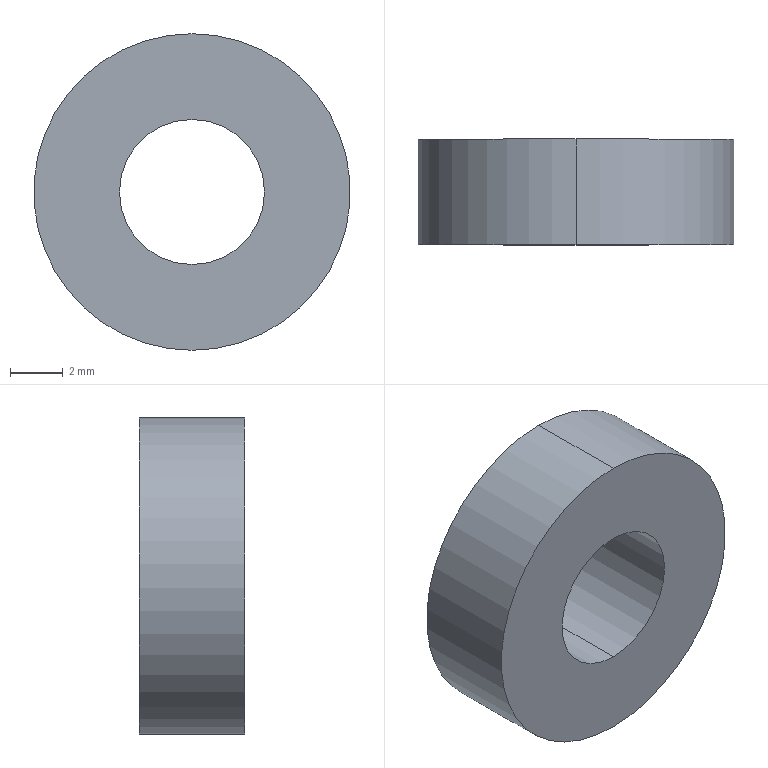Part | STEP file | PN_0026 lifting mechanism plate_Default | 1 solid | 6 faces | box 12 x 4 x 12 mm | volume 357.356 mm3 | cylinder 4 | plane 2 | commonest cylinder face diameters 5.5 x2 12 x2
STEP:
#1=CARTESIAN_POINT('',(0.,0.,0.));
#2=DIRECTION('',(0.,0.,1.));
#3=DIRECTION('',(1.,0.,0.));
#4=AXIS2_PLACEMENT_3D('',#1,#2,#3);
#5=CARTESIAN_POINT('',(0.,4.,-2.75));
#6=VERTEX_POINT('',#5);
#7=CARTESIAN_POINT('',(0.,0.,-2.75));
#8=VERTEX_POINT('',#7);
#9=CARTESIAN_POINT('',(0.,4.,-2.75));
#10=DIRECTION('',(0.,-1.,0.));
#11=VECTOR('',#10,1.);
#12=LINE('',#9,#11);
#13=CARTESIAN_POINT('',(0.,4.,0.));
#14=DIRECTION('',(0.,-1.,0.));
#15=DIRECTION('',(0.,0.,-1.));
#16=AXIS2_PLACEMENT_3D('',#13,#14,#15);
#17=CYLINDRICAL_SURFACE('',#16,2.75);
#18=CARTESIAN_POINT('',(6.283,0.));
#19=DIRECTION('',(0.,1.));
#20=VECTOR('',#19,1.);
#21=LINE('',#18,#20);
#22=(GEOMETRIC_REPRESENTATION_CONTEXT(2)PARAMETRIC_REPRESENTATION_CONTEXT()REPRESENTATION_CONTEXT('',''));
#23=DEFINITIONAL_REPRESENTATION('',(#21),#22);
#24=PCURVE('',#17,#23);
#25=CARTESIAN_POINT('',(0.,4.,0.));
#26=DIRECTION('',(0.,-1.,0.));
#27=DIRECTION('',(0.,0.,-1.));
#28=AXIS2_PLACEMENT_3D('',#25,#26,#27);
#29=CYLINDRICAL_SURFACE('',#28,2.75);
#30=CARTESIAN_POINT('',(0.,0.));
#31=DIRECTION('',(0.,1.));
#32=VECTOR('',#31,1.);
#33=LINE('',#30,#32);
#34=(GEOMETRIC_REPRESENTATION_CONTEXT(2)PARAMETRIC_REPRESENTATION_CONTEXT()REPRESENTATION_CONTEXT('',''));
#35=DEFINITIONAL_REPRESENTATION('',(#33),#34);
#36=PCURVE('',#29,#35);
#37=SURFACE_CURVE('',#12,(#24,#36),.PCURVE_S1.);
#38=EDGE_CURVE('',#6,#8,#37,.T.);
#39=ORIENTED_EDGE('',*,*,#38,.T.);
#40=CARTESIAN_POINT('',(0.,0.,2.75));
#41=VERTEX_POINT('',#40);
#42=CARTESIAN_POINT('',(0.,0.,0.));
#43=DIRECTION('',(0.,1.,0.));
#44=DIRECTION('',(0.,0.,1.));
#45=AXIS2_PLACEMENT_3D('',#42,#43,#44);
#46=CIRCLE('',#45,2.75);
#47=CARTESIAN_POINT('',(9.425,4.));
#48=DIRECTION('',(-1.,0.));
#49=VECTOR('',#48,1.);
#50=LINE('',#47,#49);
#51=(GEOMETRIC_REPRESENTATION_CONTEXT(2)PARAMETRIC_REPRESENTATION_CONTEXT()REPRESENTATION_CONTEXT('',''));
#52=DEFINITIONAL_REPRESENTATION('',(#50),#51);
#53=PCURVE('',#17,#52);
#54=CARTESIAN_POINT('',(0.,0.,0.));
#55=DIRECTION('',(0.,1.,0.));
#56=DIRECTION('',(0.,0.,1.));
#57=AXIS2_PLACEMENT_3D('',#54,#55,#56);
#58=PLANE('',#57);
#59=CARTESIAN_POINT('',(0.,0.));
#60=DIRECTION('',(1.,0.));
#61=AXIS2_PLACEMENT_2D('',#59,#60);
#62=CIRCLE('',#61,2.75);
#63=(GEOMETRIC_REPRESENTATION_CONTEXT(2)PARAMETRIC_REPRESENTATION_CONTEXT()REPRESENTATION_CONTEXT('',''));
#64=DEFINITIONAL_REPRESENTATION('',(#62),#63);
#65=PCURVE('',#58,#64);
#66=SURFACE_CURVE('',#46,(#53,#65),.PCURVE_S1.);
#67=EDGE_CURVE('',#8,#41,#66,.T.);
#68=ORIENTED_EDGE('',*,*,#67,.T.);
#69=CARTESIAN_POINT('',(0.,4.,2.75));
#70=VERTEX_POINT('',#69);
#71=CARTESIAN_POINT('',(0.,4.,2.75));
#72=DIRECTION('',(0.,-1.,0.));
#73=VECTOR('',#72,1.);
#74=LINE('',#71,#73);
#75=CARTESIAN_POINT('',(3.142,0.));
#76=DIRECTION('',(0.,1.));
#77=VECTOR('',#76,1.);
#78=LINE('',#75,#77);
#79=(GEOMETRIC_REPRESENTATION_CONTEXT(2)PARAMETRIC_REPRESENTATION_CONTEXT()REPRESENTATION_CONTEXT('',''));
#80=DEFINITIONAL_REPRESENTATION('',(#78),#79);
#81=PCURVE('',#17,#80);
#82=CARTESIAN_POINT('',(3.142,0.));
#83=DIRECTION('',(0.,1.));
#84=VECTOR('',#83,1.);
#85=LINE('',#82,#84);
#86=(GEOMETRIC_REPRESENTATION_CONTEXT(2)PARAMETRIC_REPRESENTATION_CONTEXT()REPRESENTATION_CONTEXT('',''));
#87=DEFINITIONAL_REPRESENTATION('',(#85),#86);
#88=PCURVE('',#29,#87);
#89=SURFACE_CURVE('',#74,(#81,#88),.PCURVE_S1.);
#90=EDGE_CURVE('',#70,#41,#89,.T.);
#91=ORIENTED_EDGE('',*,*,#90,.F.);
#92=CARTESIAN_POINT('',(0.,4.,0.));
#93=DIRECTION('',(0.,1.,0.));
#94=DIRECTION('',(0.,0.,1.));
#95=AXIS2_PLACEMENT_3D('',#92,#93,#94);
#96=CIRCLE('',#95,2.75);
#97=CARTESIAN_POINT('',(9.425,0.));
#98=DIRECTION('',(-1.,0.));
#99=VECTOR('',#98,1.);
#100=LINE('',#97,#99);
#101=(GEOMETRIC_REPRESENTATION_CONTEXT(2)PARAMETRIC_REPRESENTATION_CONTEXT()REPRESENTATION_CONTEXT('',''));
#102=DEFINITIONAL_REPRESENTATION('',(#100),#101);
#103=PCURVE('',#17,#102);
#104=CARTESIAN_POINT('',(0.,4.,0.));
#105=DIRECTION('',(0.,1.,0.));
#106=DIRECTION('',(0.,0.,1.));
#107=AXIS2_PLACEMENT_3D('',#104,#105,#106);
#108=PLANE('',#107);
#109=CARTESIAN_POINT('',(0.,0.));
#110=DIRECTION('',(1.,0.));
#111=AXIS2_PLACEMENT_2D('',#109,#110);
#112=CIRCLE('',#111,2.75);
#113=(GEOMETRIC_REPRESENTATION_CONTEXT(2)PARAMETRIC_REPRESENTATION_CONTEXT()REPRESENTATION_CONTEXT('',''));
#114=DEFINITIONAL_REPRESENTATION('',(#112),#113);
#115=PCURVE('',#108,#114);
#116=SURFACE_CURVE('',#96,(#103,#115),.PCURVE_S1.);
#117=EDGE_CURVE('',#6,#70,#116,.T.);
#118=ORIENTED_EDGE('',*,*,#117,.F.);
#119=EDGE_LOOP('',(#39,#68,#91,#118));
#120=FACE_BOUND('',#119,.F.);
#121=ADVANCED_FACE('',(#120),#17,.F.);
#122=CARTESIAN_POINT('',(0.,4.,6.));
#123=VERTEX_POINT('',#122);
#124=CARTESIAN_POINT('',(0.,4.,-6.));
#125=VERTEX_POINT('',#124);
#126=CARTESIAN_POINT('',(0.,4.,0.));
#127=DIRECTION('',(0.,1.,0.));
#128=DIRECTION('',(0.,0.,1.));
#129=AXIS2_PLACEMENT_3D('',#126,#127,#128);
#130=CIRCLE('',#129,6.);
#131=CARTESIAN_POINT('',(0.,4.,0.));
#132=DIRECTION('',(0.,-1.,0.));
#133=DIRECTION('',(0.,0.,-1.));
#134=AXIS2_PLACEMENT_3D('',#131,#132,#133);
#135=CYLINDRICAL_SURFACE('',#134,6.);
#136=CARTESIAN_POINT('',(3.142,0.));
#137=DIRECTION('',(-1.,0.));
#138=VECTOR('',#137,1.);
#139=LINE('',#136,#138);
#140=(GEOMETRIC_REPRESENTATION_CONTEXT(2)PARAMETRIC_REPRESENTATION_CONTEXT()REPRESENTATION_CONTEXT('',''));
#141=DEFINITIONAL_REPRESENTATION('',(#139),#140);
#142=PCURVE('',#135,#141);
#143=CARTESIAN_POINT('',(0.,0.));
#144=DIRECTION('',(1.,0.));
#145=AXIS2_PLACEMENT_2D('',#143,#144);
#146=CIRCLE('',#145,6.);
#147=(GEOMETRIC_REPRESENTATION_CONTEXT(2)PARAMETRIC_REPRESENTATION_CONTEXT()REPRESENTATION_CONTEXT('',''));
#148=DEFINITIONAL_REPRESENTATION('',(#146),#147);
#149=PCURVE('',#108,#148);
#150=SURFACE_CURVE('',#130,(#142,#149),.PCURVE_S1.);
#151=EDGE_CURVE('',#123,#125,#150,.T.);
#152=ORIENTED_EDGE('',*,*,#151,.F.);
#153=CARTESIAN_POINT('',(0.,0.,6.));
#154=VERTEX_POINT('',#153);
#155=CARTESIAN_POINT('',(0.,4.,6.));
#156=DIRECTION('',(0.,-1.,0.));
#157=VECTOR('',#156,1.);
#158=LINE('',#155,#157);
#159=CARTESIAN_POINT('',(3.142,0.));
#160=DIRECTION('',(0.,1.));
#161=VECTOR('',#160,1.);
#162=LINE('',#159,#161);
#163=(GEOMETRIC_REPRESENTATION_CONTEXT(2)PARAMETRIC_REPRESENTATION_CONTEXT()REPRESENTATION_CONTEXT('',''));
#164=DEFINITIONAL_REPRESENTATION('',(#162),#163);
#165=PCURVE('',#135,#164);
#166=CARTESIAN_POINT('',(0.,4.,0.));
#167=DIRECTION('',(0.,-1.,0.));
#168=DIRECTION('',(0.,0.,-1.));
#169=AXIS2_PLACEMENT_3D('',#166,#167,#168);
#170=CYLINDRICAL_SURFACE('',#169,6.);
#171=CARTESIAN_POINT('',(3.142,0.));
#172=DIRECTION('',(0.,1.));
#173=VECTOR('',#172,1.);
#174=LINE('',#171,#173);
#175=(GEOMETRIC_REPRESENTATION_CONTEXT(2)PARAMETRIC_REPRESENTATION_CONTEXT()REPRESENTATION_CONTEXT('',''));
#176=DEFINITIONAL_REPRESENTATION('',(#174),#175);
#177=PCURVE('',#170,#176);
#178=SURFACE_CURVE('',#158,(#165,#177),.PCURVE_S1.);
#179=EDGE_CURVE('',#123,#154,#178,.T.);
#180=ORIENTED_EDGE('',*,*,#179,.T.);
#181=CARTESIAN_POINT('',(0.,0.,-6.));
#182=VERTEX_POINT('',#181);
#183=CARTESIAN_POINT('',(0.,0.,0.));
#184=DIRECTION('',(0.,1.,0.));
#185=DIRECTION('',(0.,0.,1.));
#186=AXIS2_PLACEMENT_3D('',#183,#184,#185);
#187=CIRCLE('',#186,6.);
#188=CARTESIAN_POINT('',(3.142,4.));
#189=DIRECTION('',(-1.,0.));
#190=VECTOR('',#189,1.);
#191=LINE('',#188,#190);
#192=(GEOMETRIC_REPRESENTATION_CONTEXT(2)PARAMETRIC_REPRESENTATION_CONTEXT()REPRESENTATION_CONTEXT('',''));
#193=DEFINITIONAL_REPRESENTATION('',(#191),#192);
#194=PCURVE('',#135,#193);
#195=CARTESIAN_POINT('',(0.,0.));
#196=DIRECTION('',(1.,0.));
#197=AXIS2_PLACEMENT_2D('',#195,#196);
#198=CIRCLE('',#197,6.);
#199=(GEOMETRIC_REPRESENTATION_CONTEXT(2)PARAMETRIC_REPRESENTATION_CONTEXT()REPRESENTATION_CONTEXT('',''));
#200=DEFINITIONAL_REPRESENTATION('',(#198),#199);
#201=PCURVE('',#58,#200);
#202=SURFACE_CURVE('',#187,(#194,#201),.PCURVE_S1.);
#203=EDGE_CURVE('',#154,#182,#202,.T.);
#204=ORIENTED_EDGE('',*,*,#203,.T.);
#205=CARTESIAN_POINT('',(0.,4.,-6.));
#206=DIRECTION('',(0.,-1.,0.));
#207=VECTOR('',#206,1.);
#208=LINE('',#205,#207);
#209=CARTESIAN_POINT('',(0.,0.));
#210=DIRECTION('',(0.,1.));
#211=VECTOR('',#210,1.);
#212=LINE('',#209,#211);
#213=(GEOMETRIC_REPRESENTATION_CONTEXT(2)PARAMETRIC_REPRESENTATION_CONTEXT()REPRESENTATION_CONTEXT('',''));
#214=DEFINITIONAL_REPRESENTATION('',(#212),#213);
#215=PCURVE('',#135,#214);
#216=CARTESIAN_POINT('',(6.283,0.));
#217=DIRECTION('',(0.,1.));
#218=VECTOR('',#217,1.);
#219=LINE('',#216,#218);
#220=(GEOMETRIC_REPRESENTATION_CONTEXT(2)PARAMETRIC_REPRESENTATION_CONTEXT()REPRESENTATION_CONTEXT('',''));
#221=DEFINITIONAL_REPRESENTATION('',(#219),#220);
#222=PCURVE('',#170,#221);
#223=SURFACE_CURVE('',#208,(#215,#222),.PCURVE_S1.);
#224=EDGE_CURVE('',#125,#182,#223,.T.);
#225=ORIENTED_EDGE('',*,*,#224,.F.);
#226=EDGE_LOOP('',(#152,#180,#204,#225));
#227=FACE_BOUND('',#226,.T.);
#228=ADVANCED_FACE('',(#227),#135,.T.);
#229=CARTESIAN_POINT('',(0.,4.,0.));
#230=DIRECTION('',(0.,1.,0.));
#231=DIRECTION('',(0.,0.,1.));
#232=AXIS2_PLACEMENT_3D('',#229,#230,#231);
#233=CIRCLE('',#232,6.);
#234=CARTESIAN_POINT('',(0.,0.));
#235=DIRECTION('',(1.,0.));
#236=AXIS2_PLACEMENT_2D('',#234,#235);
#237=CIRCLE('',#236,6.);
#238=(GEOMETRIC_REPRESENTATION_CONTEXT(2)PARAMETRIC_REPRESENTATION_CONTEXT()REPRESENTATION_CONTEXT('',''));
#239=DEFINITIONAL_REPRESENTATION('',(#237),#238);
#240=PCURVE('',#108,#239);
#241=CARTESIAN_POINT('',(9.425,0.));
#242=DIRECTION('',(-1.,0.));
#243=VECTOR('',#242,1.);
#244=LINE('',#241,#243);
#245=(GEOMETRIC_REPRESENTATION_CONTEXT(2)PARAMETRIC_REPRESENTATION_CONTEXT()REPRESENTATION_CONTEXT('',''));
#246=DEFINITIONAL_REPRESENTATION('',(#244),#245);
#247=PCURVE('',#170,#246);
#248=SURFACE_CURVE('',#233,(#240,#247),.PCURVE_S1.);
#249=EDGE_CURVE('',#125,#123,#248,.T.);
#250=ORIENTED_EDGE('',*,*,#249,.T.);
#251=ORIENTED_EDGE('',*,*,#151,.T.);
#252=EDGE_LOOP('',(#250,#251));
#253=FACE_BOUND('',#252,.T.);
#254=ORIENTED_EDGE('',*,*,#117,.F.);
#255=CARTESIAN_POINT('',(0.,4.,0.));
#256=DIRECTION('',(0.,1.,0.));
#257=DIRECTION('',(0.,0.,1.));
#258=AXIS2_PLACEMENT_3D('',#255,#256,#257);
#259=CIRCLE('',#258,2.75);
#260=CARTESIAN_POINT('',(0.,0.));
#261=DIRECTION('',(1.,0.));
#262=AXIS2_PLACEMENT_2D('',#260,#261);
#263=CIRCLE('',#262,2.75);
#264=(GEOMETRIC_REPRESENTATION_CONTEXT(2)PARAMETRIC_REPRESENTATION_CONTEXT()REPRESENTATION_CONTEXT('',''));
#265=DEFINITIONAL_REPRESENTATION('',(#263),#264);
#266=PCURVE('',#108,#265);
#267=CARTESIAN_POINT('',(3.142,0.));
#268=DIRECTION('',(-1.,0.));
#269=VECTOR('',#268,1.);
#270=LINE('',#267,#269);
#271=(GEOMETRIC_REPRESENTATION_CONTEXT(2)PARAMETRIC_REPRESENTATION_CONTEXT()REPRESENTATION_CONTEXT('',''));
#272=DEFINITIONAL_REPRESENTATION('',(#270),#271);
#273=PCURVE('',#29,#272);
#274=SURFACE_CURVE('',#259,(#266,#273),.PCURVE_S1.);
#275=EDGE_CURVE('',#70,#6,#274,.T.);
#276=ORIENTED_EDGE('',*,*,#275,.F.);
#277=EDGE_LOOP('',(#254,#276));
#278=FACE_BOUND('',#277,.T.);
#279=ADVANCED_FACE('',(#253,#278),#108,.T.);
#280=CARTESIAN_POINT('',(0.,0.,0.));
#281=DIRECTION('',(0.,1.,0.));
#282=DIRECTION('',(0.,0.,1.));
#283=AXIS2_PLACEMENT_3D('',#280,#281,#282);
#284=CIRCLE('',#283,6.);
#285=CARTESIAN_POINT('',(0.,0.));
#286=DIRECTION('',(1.,0.));
#287=AXIS2_PLACEMENT_2D('',#285,#286);
#288=CIRCLE('',#287,6.);
#289=(GEOMETRIC_REPRESENTATION_CONTEXT(2)PARAMETRIC_REPRESENTATION_CONTEXT()REPRESENTATION_CONTEXT('',''));
#290=DEFINITIONAL_REPRESENTATION('',(#288),#289);
#291=PCURVE('',#58,#290);
#292=CARTESIAN_POINT('',(9.425,4.));
#293=DIRECTION('',(-1.,0.));
#294=VECTOR('',#293,1.);
#295=LINE('',#292,#294);
#296=(GEOMETRIC_REPRESENTATION_CONTEXT(2)PARAMETRIC_REPRESENTATION_CONTEXT()REPRESENTATION_CONTEXT('',''));
#297=DEFINITIONAL_REPRESENTATION('',(#295),#296);
#298=PCURVE('',#170,#297);
#299=SURFACE_CURVE('',#284,(#291,#298),.PCURVE_S1.);
#300=EDGE_CURVE('',#182,#154,#299,.T.);
#301=ORIENTED_EDGE('',*,*,#300,.F.);
#302=ORIENTED_EDGE('',*,*,#203,.F.);
#303=EDGE_LOOP('',(#301,#302));
#304=FACE_BOUND('',#303,.T.);
#305=ORIENTED_EDGE('',*,*,#67,.T.);
#306=CARTESIAN_POINT('',(0.,0.,0.));
#307=DIRECTION('',(0.,1.,0.));
#308=DIRECTION('',(0.,0.,1.));
#309=AXIS2_PLACEMENT_3D('',#306,#307,#308);
#310=CIRCLE('',#309,2.75);
#311=CARTESIAN_POINT('',(0.,0.));
#312=DIRECTION('',(1.,0.));
#313=AXIS2_PLACEMENT_2D('',#311,#312);
#314=CIRCLE('',#313,2.75);
#315=(GEOMETRIC_REPRESENTATION_CONTEXT(2)PARAMETRIC_REPRESENTATION_CONTEXT()REPRESENTATION_CONTEXT('',''));
#316=DEFINITIONAL_REPRESENTATION('',(#314),#315);
#317=PCURVE('',#58,#316);
#318=CARTESIAN_POINT('',(3.142,4.));
#319=DIRECTION('',(-1.,0.));
#320=VECTOR('',#319,1.);
#321=LINE('',#318,#320);
#322=(GEOMETRIC_REPRESENTATION_CONTEXT(2)PARAMETRIC_REPRESENTATION_CONTEXT()REPRESENTATION_CONTEXT('',''));
#323=DEFINITIONAL_REPRESENTATION('',(#321),#322);
#324=PCURVE('',#29,#323);
#325=SURFACE_CURVE('',#310,(#317,#324),.PCURVE_S1.);
#326=EDGE_CURVE('',#41,#8,#325,.T.);
#327=ORIENTED_EDGE('',*,*,#326,.T.);
#328=EDGE_LOOP('',(#305,#327));
#329=FACE_BOUND('',#328,.T.);
#330=ADVANCED_FACE('',(#304,#329),#58,.F.);
#331=ORIENTED_EDGE('',*,*,#179,.F.);
#332=ORIENTED_EDGE('',*,*,#249,.F.);
#333=ORIENTED_EDGE('',*,*,#224,.T.);
#334=ORIENTED_EDGE('',*,*,#300,.T.);
#335=EDGE_LOOP('',(#331,#332,#333,#334));
#336=FACE_BOUND('',#335,.T.);
#337=ADVANCED_FACE('',(#336),#170,.T.);
#338=ORIENTED_EDGE('',*,*,#326,.T.);
#339=ORIENTED_EDGE('',*,*,#38,.F.);
#340=ORIENTED_EDGE('',*,*,#275,.F.);
#341=ORIENTED_EDGE('',*,*,#90,.T.);
#342=EDGE_LOOP('',(#338,#339,#340,#341));
#343=FACE_BOUND('',#342,.F.);
#344=ADVANCED_FACE('',(#343),#29,.F.);
#345=CLOSED_SHELL('',(#121,#228,#279,#330,#337,#344));
#346=MANIFOLD_SOLID_BREP('',#345);
#347=(LENGTH_UNIT()NAMED_UNIT(*)SI_UNIT(.MILLI.,.METRE.));
#348=UNCERTAINTY_MEASURE_WITH_UNIT(LENGTH_MEASURE(0.0000001),#347,'','');
#349=(NAMED_UNIT(*)PLANE_ANGLE_UNIT()SI_UNIT($,.RADIAN.));
#350=(NAMED_UNIT(*)SI_UNIT($,.STERADIAN.)SOLID_ANGLE_UNIT());
#351=(GEOMETRIC_REPRESENTATION_CONTEXT(3)GLOBAL_UNCERTAINTY_ASSIGNED_CONTEXT((#348))GLOBAL_UNIT_ASSIGNED_CONTEXT((#347,#349,#350))REPRESENTATION_CONTEXT('',''));
#352=ADVANCED_BREP_SHAPE_REPRESENTATION('',(#4,#346),#351);